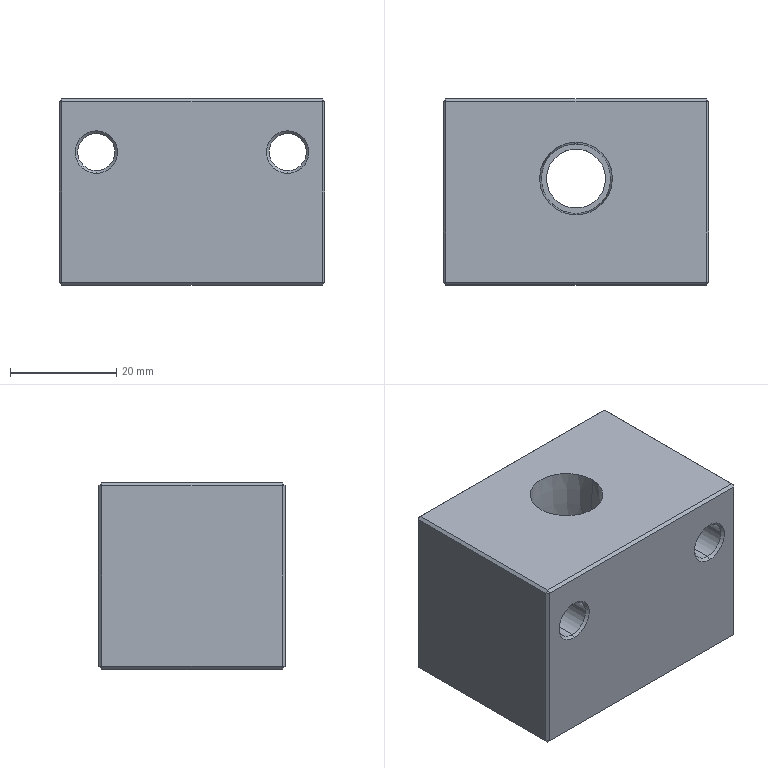Part | STEP file | OP10-013_junction block (D) | 1 solid | 46 faces | box 50 x 35 x 35 mm | volume 54198 mm3 | plane 28 | cone 12 | cylinder 6 | commonest cylinder face diameters 7 x4 11.125 x2